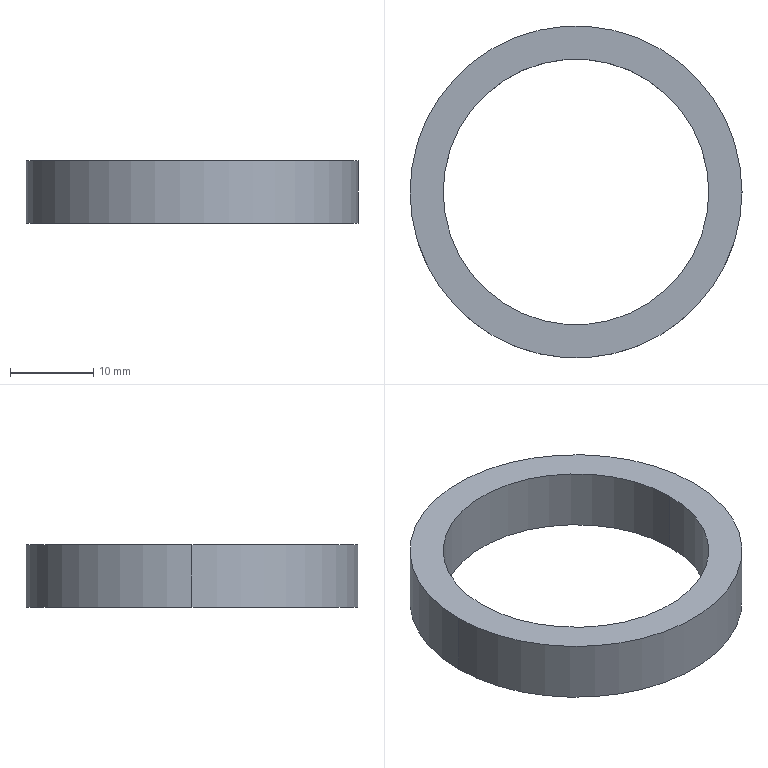Part | STEP file | BU-A15a | 1 solid | 6 faces | box 40 x 40 x 7.5 mm | volume 3393 mm3 | cylinder 4 | plane 2 | commonest cylinder face diameters 32 x2 40 x2
STEP:
#1=CARTESIAN_POINT('',(0.,0.,0.));
#2=DIRECTION('',(0.,0.,1.));
#3=DIRECTION('',(1.,0.,0.));
#4=AXIS2_PLACEMENT_3D('',#1,#2,#3);
#5=CARTESIAN_POINT('',(-16.,0.,7.5));
#6=VERTEX_POINT('',#5);
#7=CARTESIAN_POINT('',(-16.,0.,0.));
#8=VERTEX_POINT('',#7);
#9=CARTESIAN_POINT('',(-16.,0.,7.5));
#10=DIRECTION('',(0.,0.,-1.));
#11=VECTOR('',#10,1.);
#12=LINE('',#9,#11);
#13=CARTESIAN_POINT('',(0.,0.,7.5));
#14=DIRECTION('',(0.,0.,-1.));
#15=DIRECTION('',(-1.,0.,0.));
#16=AXIS2_PLACEMENT_3D('',#13,#14,#15);
#17=CYLINDRICAL_SURFACE('',#16,16.);
#18=CARTESIAN_POINT('',(6.283,0.));
#19=DIRECTION('',(0.,1.));
#20=VECTOR('',#19,1.);
#21=LINE('',#18,#20);
#22=(GEOMETRIC_REPRESENTATION_CONTEXT(2)PARAMETRIC_REPRESENTATION_CONTEXT()REPRESENTATION_CONTEXT('',''));
#23=DEFINITIONAL_REPRESENTATION('',(#21),#22);
#24=PCURVE('',#17,#23);
#25=CARTESIAN_POINT('',(0.,0.,7.5));
#26=DIRECTION('',(0.,0.,-1.));
#27=DIRECTION('',(-1.,0.,0.));
#28=AXIS2_PLACEMENT_3D('',#25,#26,#27);
#29=CYLINDRICAL_SURFACE('',#28,16.);
#30=CARTESIAN_POINT('',(0.,0.));
#31=DIRECTION('',(0.,1.));
#32=VECTOR('',#31,1.);
#33=LINE('',#30,#32);
#34=(GEOMETRIC_REPRESENTATION_CONTEXT(2)PARAMETRIC_REPRESENTATION_CONTEXT()REPRESENTATION_CONTEXT('',''));
#35=DEFINITIONAL_REPRESENTATION('',(#33),#34);
#36=PCURVE('',#29,#35);
#37=SURFACE_CURVE('',#12,(#24,#36),.PCURVE_S1.);
#38=EDGE_CURVE('',#6,#8,#37,.T.);
#39=ORIENTED_EDGE('',*,*,#38,.T.);
#40=CARTESIAN_POINT('',(16.,0.,0.));
#41=VERTEX_POINT('',#40);
#42=CARTESIAN_POINT('',(0.,0.,0.));
#43=DIRECTION('',(0.,0.,1.));
#44=DIRECTION('',(1.,0.,0.));
#45=AXIS2_PLACEMENT_3D('',#42,#43,#44);
#46=CIRCLE('',#45,16.);
#47=CARTESIAN_POINT('',(9.425,7.5));
#48=DIRECTION('',(-1.,0.));
#49=VECTOR('',#48,1.);
#50=LINE('',#47,#49);
#51=(GEOMETRIC_REPRESENTATION_CONTEXT(2)PARAMETRIC_REPRESENTATION_CONTEXT()REPRESENTATION_CONTEXT('',''));
#52=DEFINITIONAL_REPRESENTATION('',(#50),#51);
#53=PCURVE('',#17,#52);
#54=CARTESIAN_POINT('',(0.,0.,0.));
#55=DIRECTION('',(0.,0.,1.));
#56=DIRECTION('',(1.,0.,0.));
#57=AXIS2_PLACEMENT_3D('',#54,#55,#56);
#58=PLANE('',#57);
#59=CARTESIAN_POINT('',(0.,0.));
#60=DIRECTION('',(1.,0.));
#61=AXIS2_PLACEMENT_2D('',#59,#60);
#62=CIRCLE('',#61,16.);
#63=(GEOMETRIC_REPRESENTATION_CONTEXT(2)PARAMETRIC_REPRESENTATION_CONTEXT()REPRESENTATION_CONTEXT('',''));
#64=DEFINITIONAL_REPRESENTATION('',(#62),#63);
#65=PCURVE('',#58,#64);
#66=SURFACE_CURVE('',#46,(#53,#65),.PCURVE_S1.);
#67=EDGE_CURVE('',#8,#41,#66,.T.);
#68=ORIENTED_EDGE('',*,*,#67,.T.);
#69=CARTESIAN_POINT('',(16.,0.,7.5));
#70=VERTEX_POINT('',#69);
#71=CARTESIAN_POINT('',(16.,0.,7.5));
#72=DIRECTION('',(0.,0.,-1.));
#73=VECTOR('',#72,1.);
#74=LINE('',#71,#73);
#75=CARTESIAN_POINT('',(3.142,0.));
#76=DIRECTION('',(0.,1.));
#77=VECTOR('',#76,1.);
#78=LINE('',#75,#77);
#79=(GEOMETRIC_REPRESENTATION_CONTEXT(2)PARAMETRIC_REPRESENTATION_CONTEXT()REPRESENTATION_CONTEXT('',''));
#80=DEFINITIONAL_REPRESENTATION('',(#78),#79);
#81=PCURVE('',#17,#80);
#82=CARTESIAN_POINT('',(3.142,0.));
#83=DIRECTION('',(0.,1.));
#84=VECTOR('',#83,1.);
#85=LINE('',#82,#84);
#86=(GEOMETRIC_REPRESENTATION_CONTEXT(2)PARAMETRIC_REPRESENTATION_CONTEXT()REPRESENTATION_CONTEXT('',''));
#87=DEFINITIONAL_REPRESENTATION('',(#85),#86);
#88=PCURVE('',#29,#87);
#89=SURFACE_CURVE('',#74,(#81,#88),.PCURVE_S1.);
#90=EDGE_CURVE('',#70,#41,#89,.T.);
#91=ORIENTED_EDGE('',*,*,#90,.F.);
#92=CARTESIAN_POINT('',(0.,0.,7.5));
#93=DIRECTION('',(0.,0.,1.));
#94=DIRECTION('',(1.,0.,0.));
#95=AXIS2_PLACEMENT_3D('',#92,#93,#94);
#96=CIRCLE('',#95,16.);
#97=CARTESIAN_POINT('',(9.425,0.));
#98=DIRECTION('',(-1.,0.));
#99=VECTOR('',#98,1.);
#100=LINE('',#97,#99);
#101=(GEOMETRIC_REPRESENTATION_CONTEXT(2)PARAMETRIC_REPRESENTATION_CONTEXT()REPRESENTATION_CONTEXT('',''));
#102=DEFINITIONAL_REPRESENTATION('',(#100),#101);
#103=PCURVE('',#17,#102);
#104=CARTESIAN_POINT('',(0.,0.,7.5));
#105=DIRECTION('',(0.,0.,1.));
#106=DIRECTION('',(1.,0.,0.));
#107=AXIS2_PLACEMENT_3D('',#104,#105,#106);
#108=PLANE('',#107);
#109=CARTESIAN_POINT('',(0.,0.));
#110=DIRECTION('',(1.,0.));
#111=AXIS2_PLACEMENT_2D('',#109,#110);
#112=CIRCLE('',#111,16.);
#113=(GEOMETRIC_REPRESENTATION_CONTEXT(2)PARAMETRIC_REPRESENTATION_CONTEXT()REPRESENTATION_CONTEXT('',''));
#114=DEFINITIONAL_REPRESENTATION('',(#112),#113);
#115=PCURVE('',#108,#114);
#116=SURFACE_CURVE('',#96,(#103,#115),.PCURVE_S1.);
#117=EDGE_CURVE('',#6,#70,#116,.T.);
#118=ORIENTED_EDGE('',*,*,#117,.F.);
#119=EDGE_LOOP('',(#39,#68,#91,#118));
#120=FACE_BOUND('',#119,.F.);
#121=ADVANCED_FACE('',(#120),#17,.F.);
#122=CARTESIAN_POINT('',(20.,0.,7.5));
#123=VERTEX_POINT('',#122);
#124=CARTESIAN_POINT('',(-20.,0.,7.5));
#125=VERTEX_POINT('',#124);
#126=CARTESIAN_POINT('',(0.,0.,7.5));
#127=DIRECTION('',(0.,0.,1.));
#128=DIRECTION('',(1.,0.,0.));
#129=AXIS2_PLACEMENT_3D('',#126,#127,#128);
#130=CIRCLE('',#129,20.);
#131=CARTESIAN_POINT('',(0.,0.,7.5));
#132=DIRECTION('',(0.,0.,-1.));
#133=DIRECTION('',(-1.,0.,0.));
#134=AXIS2_PLACEMENT_3D('',#131,#132,#133);
#135=CYLINDRICAL_SURFACE('',#134,20.);
#136=CARTESIAN_POINT('',(3.142,0.));
#137=DIRECTION('',(-1.,0.));
#138=VECTOR('',#137,1.);
#139=LINE('',#136,#138);
#140=(GEOMETRIC_REPRESENTATION_CONTEXT(2)PARAMETRIC_REPRESENTATION_CONTEXT()REPRESENTATION_CONTEXT('',''));
#141=DEFINITIONAL_REPRESENTATION('',(#139),#140);
#142=PCURVE('',#135,#141);
#143=CARTESIAN_POINT('',(0.,0.));
#144=DIRECTION('',(1.,0.));
#145=AXIS2_PLACEMENT_2D('',#143,#144);
#146=CIRCLE('',#145,20.);
#147=(GEOMETRIC_REPRESENTATION_CONTEXT(2)PARAMETRIC_REPRESENTATION_CONTEXT()REPRESENTATION_CONTEXT('',''));
#148=DEFINITIONAL_REPRESENTATION('',(#146),#147);
#149=PCURVE('',#108,#148);
#150=SURFACE_CURVE('',#130,(#142,#149),.PCURVE_S1.);
#151=EDGE_CURVE('',#123,#125,#150,.T.);
#152=ORIENTED_EDGE('',*,*,#151,.F.);
#153=CARTESIAN_POINT('',(20.,0.,0.));
#154=VERTEX_POINT('',#153);
#155=CARTESIAN_POINT('',(20.,0.,7.5));
#156=DIRECTION('',(0.,0.,-1.));
#157=VECTOR('',#156,1.);
#158=LINE('',#155,#157);
#159=CARTESIAN_POINT('',(3.142,0.));
#160=DIRECTION('',(0.,1.));
#161=VECTOR('',#160,1.);
#162=LINE('',#159,#161);
#163=(GEOMETRIC_REPRESENTATION_CONTEXT(2)PARAMETRIC_REPRESENTATION_CONTEXT()REPRESENTATION_CONTEXT('',''));
#164=DEFINITIONAL_REPRESENTATION('',(#162),#163);
#165=PCURVE('',#135,#164);
#166=CARTESIAN_POINT('',(0.,0.,7.5));
#167=DIRECTION('',(0.,0.,-1.));
#168=DIRECTION('',(-1.,0.,0.));
#169=AXIS2_PLACEMENT_3D('',#166,#167,#168);
#170=CYLINDRICAL_SURFACE('',#169,20.);
#171=CARTESIAN_POINT('',(3.142,0.));
#172=DIRECTION('',(0.,1.));
#173=VECTOR('',#172,1.);
#174=LINE('',#171,#173);
#175=(GEOMETRIC_REPRESENTATION_CONTEXT(2)PARAMETRIC_REPRESENTATION_CONTEXT()REPRESENTATION_CONTEXT('',''));
#176=DEFINITIONAL_REPRESENTATION('',(#174),#175);
#177=PCURVE('',#170,#176);
#178=SURFACE_CURVE('',#158,(#165,#177),.PCURVE_S1.);
#179=EDGE_CURVE('',#123,#154,#178,.T.);
#180=ORIENTED_EDGE('',*,*,#179,.T.);
#181=CARTESIAN_POINT('',(-20.,0.,0.));
#182=VERTEX_POINT('',#181);
#183=CARTESIAN_POINT('',(0.,0.,0.));
#184=DIRECTION('',(0.,0.,1.));
#185=DIRECTION('',(1.,0.,0.));
#186=AXIS2_PLACEMENT_3D('',#183,#184,#185);
#187=CIRCLE('',#186,20.);
#188=CARTESIAN_POINT('',(3.142,7.5));
#189=DIRECTION('',(-1.,0.));
#190=VECTOR('',#189,1.);
#191=LINE('',#188,#190);
#192=(GEOMETRIC_REPRESENTATION_CONTEXT(2)PARAMETRIC_REPRESENTATION_CONTEXT()REPRESENTATION_CONTEXT('',''));
#193=DEFINITIONAL_REPRESENTATION('',(#191),#192);
#194=PCURVE('',#135,#193);
#195=CARTESIAN_POINT('',(0.,0.));
#196=DIRECTION('',(1.,0.));
#197=AXIS2_PLACEMENT_2D('',#195,#196);
#198=CIRCLE('',#197,20.);
#199=(GEOMETRIC_REPRESENTATION_CONTEXT(2)PARAMETRIC_REPRESENTATION_CONTEXT()REPRESENTATION_CONTEXT('',''));
#200=DEFINITIONAL_REPRESENTATION('',(#198),#199);
#201=PCURVE('',#58,#200);
#202=SURFACE_CURVE('',#187,(#194,#201),.PCURVE_S1.);
#203=EDGE_CURVE('',#154,#182,#202,.T.);
#204=ORIENTED_EDGE('',*,*,#203,.T.);
#205=CARTESIAN_POINT('',(-20.,0.,7.5));
#206=DIRECTION('',(0.,0.,-1.));
#207=VECTOR('',#206,1.);
#208=LINE('',#205,#207);
#209=CARTESIAN_POINT('',(0.,0.));
#210=DIRECTION('',(0.,1.));
#211=VECTOR('',#210,1.);
#212=LINE('',#209,#211);
#213=(GEOMETRIC_REPRESENTATION_CONTEXT(2)PARAMETRIC_REPRESENTATION_CONTEXT()REPRESENTATION_CONTEXT('',''));
#214=DEFINITIONAL_REPRESENTATION('',(#212),#213);
#215=PCURVE('',#135,#214);
#216=CARTESIAN_POINT('',(6.283,0.));
#217=DIRECTION('',(0.,1.));
#218=VECTOR('',#217,1.);
#219=LINE('',#216,#218);
#220=(GEOMETRIC_REPRESENTATION_CONTEXT(2)PARAMETRIC_REPRESENTATION_CONTEXT()REPRESENTATION_CONTEXT('',''));
#221=DEFINITIONAL_REPRESENTATION('',(#219),#220);
#222=PCURVE('',#170,#221);
#223=SURFACE_CURVE('',#208,(#215,#222),.PCURVE_S1.);
#224=EDGE_CURVE('',#125,#182,#223,.T.);
#225=ORIENTED_EDGE('',*,*,#224,.F.);
#226=EDGE_LOOP('',(#152,#180,#204,#225));
#227=FACE_BOUND('',#226,.T.);
#228=ADVANCED_FACE('',(#227),#135,.T.);
#229=CARTESIAN_POINT('',(0.,0.,7.5));
#230=DIRECTION('',(0.,0.,1.));
#231=DIRECTION('',(1.,0.,0.));
#232=AXIS2_PLACEMENT_3D('',#229,#230,#231);
#233=CIRCLE('',#232,20.);
#234=CARTESIAN_POINT('',(0.,0.));
#235=DIRECTION('',(1.,0.));
#236=AXIS2_PLACEMENT_2D('',#234,#235);
#237=CIRCLE('',#236,20.);
#238=(GEOMETRIC_REPRESENTATION_CONTEXT(2)PARAMETRIC_REPRESENTATION_CONTEXT()REPRESENTATION_CONTEXT('',''));
#239=DEFINITIONAL_REPRESENTATION('',(#237),#238);
#240=PCURVE('',#108,#239);
#241=CARTESIAN_POINT('',(9.425,0.));
#242=DIRECTION('',(-1.,0.));
#243=VECTOR('',#242,1.);
#244=LINE('',#241,#243);
#245=(GEOMETRIC_REPRESENTATION_CONTEXT(2)PARAMETRIC_REPRESENTATION_CONTEXT()REPRESENTATION_CONTEXT('',''));
#246=DEFINITIONAL_REPRESENTATION('',(#244),#245);
#247=PCURVE('',#170,#246);
#248=SURFACE_CURVE('',#233,(#240,#247),.PCURVE_S1.);
#249=EDGE_CURVE('',#125,#123,#248,.T.);
#250=ORIENTED_EDGE('',*,*,#249,.T.);
#251=ORIENTED_EDGE('',*,*,#151,.T.);
#252=EDGE_LOOP('',(#250,#251));
#253=FACE_BOUND('',#252,.T.);
#254=ORIENTED_EDGE('',*,*,#117,.F.);
#255=CARTESIAN_POINT('',(0.,0.,7.5));
#256=DIRECTION('',(0.,0.,1.));
#257=DIRECTION('',(1.,0.,0.));
#258=AXIS2_PLACEMENT_3D('',#255,#256,#257);
#259=CIRCLE('',#258,16.);
#260=CARTESIAN_POINT('',(0.,0.));
#261=DIRECTION('',(1.,0.));
#262=AXIS2_PLACEMENT_2D('',#260,#261);
#263=CIRCLE('',#262,16.);
#264=(GEOMETRIC_REPRESENTATION_CONTEXT(2)PARAMETRIC_REPRESENTATION_CONTEXT()REPRESENTATION_CONTEXT('',''));
#265=DEFINITIONAL_REPRESENTATION('',(#263),#264);
#266=PCURVE('',#108,#265);
#267=CARTESIAN_POINT('',(3.142,0.));
#268=DIRECTION('',(-1.,0.));
#269=VECTOR('',#268,1.);
#270=LINE('',#267,#269);
#271=(GEOMETRIC_REPRESENTATION_CONTEXT(2)PARAMETRIC_REPRESENTATION_CONTEXT()REPRESENTATION_CONTEXT('',''));
#272=DEFINITIONAL_REPRESENTATION('',(#270),#271);
#273=PCURVE('',#29,#272);
#274=SURFACE_CURVE('',#259,(#266,#273),.PCURVE_S1.);
#275=EDGE_CURVE('',#70,#6,#274,.T.);
#276=ORIENTED_EDGE('',*,*,#275,.F.);
#277=EDGE_LOOP('',(#254,#276));
#278=FACE_BOUND('',#277,.T.);
#279=ADVANCED_FACE('',(#253,#278),#108,.T.);
#280=CARTESIAN_POINT('',(0.,0.,0.));
#281=DIRECTION('',(0.,0.,1.));
#282=DIRECTION('',(1.,0.,0.));
#283=AXIS2_PLACEMENT_3D('',#280,#281,#282);
#284=CIRCLE('',#283,20.);
#285=CARTESIAN_POINT('',(0.,0.));
#286=DIRECTION('',(1.,0.));
#287=AXIS2_PLACEMENT_2D('',#285,#286);
#288=CIRCLE('',#287,20.);
#289=(GEOMETRIC_REPRESENTATION_CONTEXT(2)PARAMETRIC_REPRESENTATION_CONTEXT()REPRESENTATION_CONTEXT('',''));
#290=DEFINITIONAL_REPRESENTATION('',(#288),#289);
#291=PCURVE('',#58,#290);
#292=CARTESIAN_POINT('',(9.425,7.5));
#293=DIRECTION('',(-1.,0.));
#294=VECTOR('',#293,1.);
#295=LINE('',#292,#294);
#296=(GEOMETRIC_REPRESENTATION_CONTEXT(2)PARAMETRIC_REPRESENTATION_CONTEXT()REPRESENTATION_CONTEXT('',''));
#297=DEFINITIONAL_REPRESENTATION('',(#295),#296);
#298=PCURVE('',#170,#297);
#299=SURFACE_CURVE('',#284,(#291,#298),.PCURVE_S1.);
#300=EDGE_CURVE('',#182,#154,#299,.T.);
#301=ORIENTED_EDGE('',*,*,#300,.F.);
#302=ORIENTED_EDGE('',*,*,#203,.F.);
#303=EDGE_LOOP('',(#301,#302));
#304=FACE_BOUND('',#303,.T.);
#305=ORIENTED_EDGE('',*,*,#67,.T.);
#306=CARTESIAN_POINT('',(0.,0.,0.));
#307=DIRECTION('',(0.,0.,1.));
#308=DIRECTION('',(1.,0.,0.));
#309=AXIS2_PLACEMENT_3D('',#306,#307,#308);
#310=CIRCLE('',#309,16.);
#311=CARTESIAN_POINT('',(0.,0.));
#312=DIRECTION('',(1.,0.));
#313=AXIS2_PLACEMENT_2D('',#311,#312);
#314=CIRCLE('',#313,16.);
#315=(GEOMETRIC_REPRESENTATION_CONTEXT(2)PARAMETRIC_REPRESENTATION_CONTEXT()REPRESENTATION_CONTEXT('',''));
#316=DEFINITIONAL_REPRESENTATION('',(#314),#315);
#317=PCURVE('',#58,#316);
#318=CARTESIAN_POINT('',(3.142,7.5));
#319=DIRECTION('',(-1.,0.));
#320=VECTOR('',#319,1.);
#321=LINE('',#318,#320);
#322=(GEOMETRIC_REPRESENTATION_CONTEXT(2)PARAMETRIC_REPRESENTATION_CONTEXT()REPRESENTATION_CONTEXT('',''));
#323=DEFINITIONAL_REPRESENTATION('',(#321),#322);
#324=PCURVE('',#29,#323);
#325=SURFACE_CURVE('',#310,(#317,#324),.PCURVE_S1.);
#326=EDGE_CURVE('',#41,#8,#325,.T.);
#327=ORIENTED_EDGE('',*,*,#326,.T.);
#328=EDGE_LOOP('',(#305,#327));
#329=FACE_BOUND('',#328,.T.);
#330=ADVANCED_FACE('',(#304,#329),#58,.F.);
#331=ORIENTED_EDGE('',*,*,#179,.F.);
#332=ORIENTED_EDGE('',*,*,#249,.F.);
#333=ORIENTED_EDGE('',*,*,#224,.T.);
#334=ORIENTED_EDGE('',*,*,#300,.T.);
#335=EDGE_LOOP('',(#331,#332,#333,#334));
#336=FACE_BOUND('',#335,.T.);
#337=ADVANCED_FACE('',(#336),#170,.T.);
#338=ORIENTED_EDGE('',*,*,#326,.T.);
#339=ORIENTED_EDGE('',*,*,#38,.F.);
#340=ORIENTED_EDGE('',*,*,#275,.F.);
#341=ORIENTED_EDGE('',*,*,#90,.T.);
#342=EDGE_LOOP('',(#338,#339,#340,#341));
#343=FACE_BOUND('',#342,.F.);
#344=ADVANCED_FACE('',(#343),#29,.F.);
#345=CLOSED_SHELL('',(#121,#228,#279,#330,#337,#344));
#346=MANIFOLD_SOLID_BREP('',#345);
#347=(LENGTH_UNIT()NAMED_UNIT(*)SI_UNIT(.MILLI.,.METRE.));
#348=UNCERTAINTY_MEASURE_WITH_UNIT(LENGTH_MEASURE(0.0000001),#347,'','');
#349=(NAMED_UNIT(*)PLANE_ANGLE_UNIT()SI_UNIT($,.RADIAN.));
#350=(NAMED_UNIT(*)SI_UNIT($,.STERADIAN.)SOLID_ANGLE_UNIT());
#351=(GEOMETRIC_REPRESENTATION_CONTEXT(3)GLOBAL_UNCERTAINTY_ASSIGNED_CONTEXT((#348))GLOBAL_UNIT_ASSIGNED_CONTEXT((#347,#349,#350))REPRESENTATION_CONTEXT('',''));
#352=ADVANCED_BREP_SHAPE_REPRESENTATION('',(#4,#346),#351);